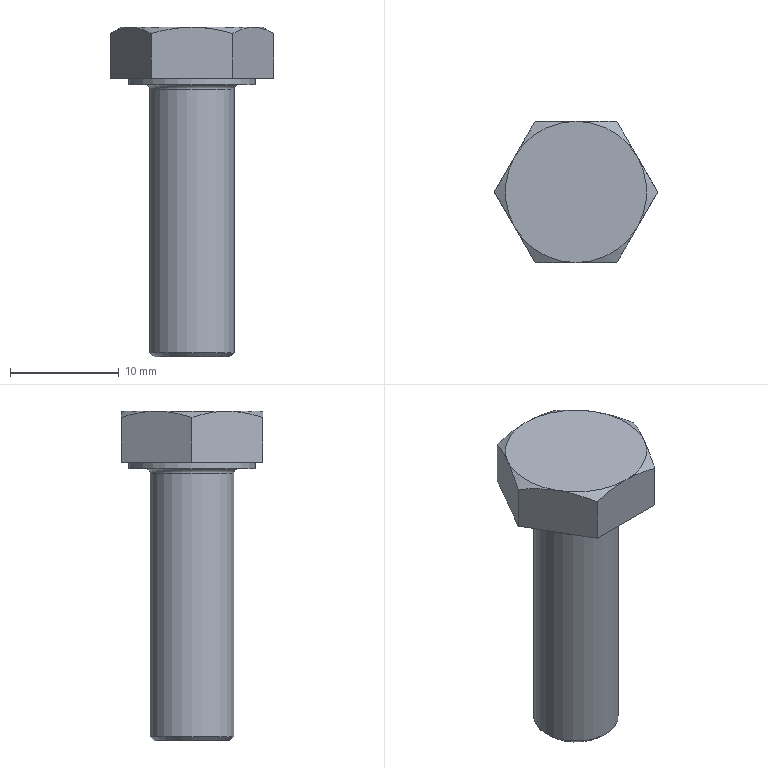Part | NX | 1 solid | 20 faces | box 15.011 x 13 x 30.3 mm | volume 1931 mm3 | plane 10 | cone 7 | cylinder 2 | torus 1 | commonest cylinder face diameters 7.76 x1 11.63 x1
STEP:
#1=CARTESIAN_POINT('',(3.753,-6.5,4.719));
#2=VERTEX_POINT('',#1);
#3=CARTESIAN_POINT('',(5.629,-3.25,5.3));
#4=VERTEX_POINT('',#3);
#5=CARTESIAN_POINT('',(3.753,-6.5,4.719));
#6=CARTESIAN_POINT('',(4.366,-5.438,5.073));
#7=CARTESIAN_POINT('',(4.989,-4.359,5.3));
#8=CARTESIAN_POINT('',(5.629,-3.25,5.3));
#9=B_SPLINE_CURVE_WITH_KNOTS('',3,(#5,#6,#7,#8),.UNSPECIFIED.,.F.,.F.,(4,4),(0.,1.),.UNSPECIFIED.);
#10=EDGE_CURVE('',#2,#4,#9,.T.);
#11=ORIENTED_EDGE('',*,*,#10,.F.);
#12=CARTESIAN_POINT('',(3.753,-6.5,0.6));
#13=VERTEX_POINT('',#12);
#14=CARTESIAN_POINT('',(3.753,-6.5,5.3));
#15=DIRECTION('',(0.,0.,-1.));
#16=VECTOR('',#15,1.);
#17=LINE('',#14,#16);
#18=EDGE_CURVE('',#2,#13,#17,.T.);
#19=ORIENTED_EDGE('',*,*,#18,.T.);
#20=CARTESIAN_POINT('',(7.506,0.,0.6));
#21=VERTEX_POINT('',#20);
#22=CARTESIAN_POINT('',(3.753,-6.5,0.6));
#23=DIRECTION('',(0.5,0.866,0.));
#24=VECTOR('',#23,1.);
#25=LINE('',#22,#24);
#26=EDGE_CURVE('',#13,#21,#25,.T.);
#27=ORIENTED_EDGE('',*,*,#26,.T.);
#28=CARTESIAN_POINT('',(7.506,0.,4.719));
#29=VERTEX_POINT('',#28);
#30=CARTESIAN_POINT('',(7.506,0.,5.3));
#31=DIRECTION('',(0.,0.,-1.));
#32=VECTOR('',#31,1.);
#33=LINE('',#30,#32);
#34=EDGE_CURVE('',#29,#21,#33,.T.);
#35=ORIENTED_EDGE('',*,*,#34,.F.);
#36=CARTESIAN_POINT('',(5.629,-3.25,5.3));
#37=CARTESIAN_POINT('',(6.27,-2.141,5.3));
#38=CARTESIAN_POINT('',(6.892,-1.062,5.073));
#39=CARTESIAN_POINT('',(7.506,0.,4.719));
#40=B_SPLINE_CURVE_WITH_KNOTS('',3,(#36,#37,#38,#39),.UNSPECIFIED.,.F.,.F.,(4,4),(0.,1.),.UNSPECIFIED.);
#41=EDGE_CURVE('',#4,#29,#40,.T.);
#42=ORIENTED_EDGE('',*,*,#41,.F.);
#43=EDGE_LOOP('',(#11,#19,#27,#35,#42));
#44=FACE_OUTER_BOUND('',#43,.T.);
#45=CARTESIAN_POINT('',(3.753,-6.5,5.3));
#46=DIRECTION('',(-0.866,0.5,0.));
#47=DIRECTION('',(0.5,0.866,0.));
#48=AXIS2_PLACEMENT_3D('',#45,#46,#47);
#49=PLANE('',#48);
#50=ADVANCED_FACE('',(#44),#49,.F.);
#51=CARTESIAN_POINT('',(5.629,3.25,5.3));
#52=VERTEX_POINT('',#51);
#53=CARTESIAN_POINT('',(7.506,0.,4.719));
#54=CARTESIAN_POINT('',(6.892,1.062,5.073));
#55=CARTESIAN_POINT('',(6.27,2.141,5.3));
#56=CARTESIAN_POINT('',(5.629,3.25,5.3));
#57=B_SPLINE_CURVE_WITH_KNOTS('',3,(#53,#54,#55,#56),.UNSPECIFIED.,.F.,.F.,(4,4),(0.,1.),.UNSPECIFIED.);
#58=EDGE_CURVE('',#29,#52,#57,.T.);
#59=ORIENTED_EDGE('',*,*,#58,.F.);
#60=ORIENTED_EDGE('',*,*,#34,.T.);
#61=CARTESIAN_POINT('',(3.753,6.5,0.6));
#62=VERTEX_POINT('',#61);
#63=CARTESIAN_POINT('',(7.506,0.,0.6));
#64=DIRECTION('',(-0.5,0.866,0.));
#65=VECTOR('',#64,1.);
#66=LINE('',#63,#65);
#67=EDGE_CURVE('',#21,#62,#66,.T.);
#68=ORIENTED_EDGE('',*,*,#67,.T.);
#69=CARTESIAN_POINT('',(3.753,6.5,4.719));
#70=VERTEX_POINT('',#69);
#71=CARTESIAN_POINT('',(3.753,6.5,5.3));
#72=DIRECTION('',(0.,0.,-1.));
#73=VECTOR('',#72,1.);
#74=LINE('',#71,#73);
#75=EDGE_CURVE('',#70,#62,#74,.T.);
#76=ORIENTED_EDGE('',*,*,#75,.F.);
#77=CARTESIAN_POINT('',(5.629,3.25,5.3));
#78=CARTESIAN_POINT('',(4.989,4.359,5.3));
#79=CARTESIAN_POINT('',(4.366,5.438,5.073));
#80=CARTESIAN_POINT('',(3.753,6.5,4.719));
#81=B_SPLINE_CURVE_WITH_KNOTS('',3,(#77,#78,#79,#80),.UNSPECIFIED.,.F.,.F.,(4,4),(0.,1.),.UNSPECIFIED.);
#82=EDGE_CURVE('',#52,#70,#81,.T.);
#83=ORIENTED_EDGE('',*,*,#82,.F.);
#84=EDGE_LOOP('',(#59,#60,#68,#76,#83));
#85=FACE_OUTER_BOUND('',#84,.T.);
#86=CARTESIAN_POINT('',(7.506,0.,5.3));
#87=DIRECTION('',(-0.866,-0.5,0.));
#88=DIRECTION('',(-0.5,0.866,0.));
#89=AXIS2_PLACEMENT_3D('',#86,#87,#88);
#90=PLANE('',#89);
#91=ADVANCED_FACE('',(#85),#90,.F.);
#92=CARTESIAN_POINT('',(0.,6.5,5.3));
#93=VERTEX_POINT('',#92);
#94=CARTESIAN_POINT('',(3.753,6.5,4.719));
#95=CARTESIAN_POINT('',(2.527,6.5,5.073));
#96=CARTESIAN_POINT('',(1.281,6.5,5.3));
#97=CARTESIAN_POINT('',(0.,6.5,5.3));
#98=B_SPLINE_CURVE_WITH_KNOTS('',3,(#94,#95,#96,#97),.UNSPECIFIED.,.F.,.F.,(4,4),(0.,1.),.UNSPECIFIED.);
#99=EDGE_CURVE('',#70,#93,#98,.T.);
#100=ORIENTED_EDGE('',*,*,#99,.F.);
#101=ORIENTED_EDGE('',*,*,#75,.T.);
#102=CARTESIAN_POINT('',(-3.753,6.5,0.6));
#103=VERTEX_POINT('',#102);
#104=CARTESIAN_POINT('',(3.753,6.5,0.6));
#105=DIRECTION('',(-1.,0.,0.));
#106=VECTOR('',#105,1.);
#107=LINE('',#104,#106);
#108=EDGE_CURVE('',#62,#103,#107,.T.);
#109=ORIENTED_EDGE('',*,*,#108,.T.);
#110=CARTESIAN_POINT('',(-3.753,6.5,4.719));
#111=VERTEX_POINT('',#110);
#112=CARTESIAN_POINT('',(-3.753,6.5,5.3));
#113=DIRECTION('',(0.,0.,-1.));
#114=VECTOR('',#113,1.);
#115=LINE('',#112,#114);
#116=EDGE_CURVE('',#111,#103,#115,.T.);
#117=ORIENTED_EDGE('',*,*,#116,.F.);
#118=CARTESIAN_POINT('',(0.,6.5,5.3));
#119=CARTESIAN_POINT('',(-1.281,6.5,5.3));
#120=CARTESIAN_POINT('',(-2.527,6.5,5.073));
#121=CARTESIAN_POINT('',(-3.753,6.5,4.719));
#122=B_SPLINE_CURVE_WITH_KNOTS('',3,(#118,#119,#120,#121),.UNSPECIFIED.,.F.,.F.,(4,4),(0.,1.),.UNSPECIFIED.);
#123=EDGE_CURVE('',#93,#111,#122,.T.);
#124=ORIENTED_EDGE('',*,*,#123,.F.);
#125=EDGE_LOOP('',(#100,#101,#109,#117,#124));
#126=FACE_OUTER_BOUND('',#125,.T.);
#127=CARTESIAN_POINT('',(3.753,6.5,5.3));
#128=DIRECTION('',(0.,-1.,0.));
#129=DIRECTION('',(-1.,0.,0.));
#130=AXIS2_PLACEMENT_3D('',#127,#128,#129);
#131=PLANE('',#130);
#132=ADVANCED_FACE('',(#126),#131,.F.);
#133=CARTESIAN_POINT('',(-5.629,3.25,5.3));
#134=VERTEX_POINT('',#133);
#135=CARTESIAN_POINT('',(-3.753,6.5,4.719));
#136=CARTESIAN_POINT('',(-4.366,5.438,5.073));
#137=CARTESIAN_POINT('',(-4.989,4.359,5.3));
#138=CARTESIAN_POINT('',(-5.629,3.25,5.3));
#139=B_SPLINE_CURVE_WITH_KNOTS('',3,(#135,#136,#137,#138),.UNSPECIFIED.,.F.,.F.,(4,4),(0.,1.),.UNSPECIFIED.);
#140=EDGE_CURVE('',#111,#134,#139,.T.);
#141=ORIENTED_EDGE('',*,*,#140,.F.);
#142=ORIENTED_EDGE('',*,*,#116,.T.);
#143=CARTESIAN_POINT('',(-7.506,0.,0.6));
#144=VERTEX_POINT('',#143);
#145=CARTESIAN_POINT('',(-3.753,6.5,0.6));
#146=DIRECTION('',(-0.5,-0.866,0.));
#147=VECTOR('',#146,1.);
#148=LINE('',#145,#147);
#149=EDGE_CURVE('',#103,#144,#148,.T.);
#150=ORIENTED_EDGE('',*,*,#149,.T.);
#151=CARTESIAN_POINT('',(-7.506,0.,4.719));
#152=VERTEX_POINT('',#151);
#153=CARTESIAN_POINT('',(-7.506,0.,5.3));
#154=DIRECTION('',(0.,0.,-1.));
#155=VECTOR('',#154,1.);
#156=LINE('',#153,#155);
#157=EDGE_CURVE('',#152,#144,#156,.T.);
#158=ORIENTED_EDGE('',*,*,#157,.F.);
#159=CARTESIAN_POINT('',(-5.629,3.25,5.3));
#160=CARTESIAN_POINT('',(-6.27,2.141,5.3));
#161=CARTESIAN_POINT('',(-6.892,1.062,5.073));
#162=CARTESIAN_POINT('',(-7.506,0.,4.719));
#163=B_SPLINE_CURVE_WITH_KNOTS('',3,(#159,#160,#161,#162),.UNSPECIFIED.,.F.,.F.,(4,4),(0.,1.),.UNSPECIFIED.);
#164=EDGE_CURVE('',#134,#152,#163,.T.);
#165=ORIENTED_EDGE('',*,*,#164,.F.);
#166=EDGE_LOOP('',(#141,#142,#150,#158,#165));
#167=FACE_OUTER_BOUND('',#166,.T.);
#168=CARTESIAN_POINT('',(-3.753,6.5,5.3));
#169=DIRECTION('',(0.866,-0.5,0.));
#170=DIRECTION('',(-0.5,-0.866,0.));
#171=AXIS2_PLACEMENT_3D('',#168,#169,#170);
#172=PLANE('',#171);
#173=ADVANCED_FACE('',(#167),#172,.F.);
#174=CARTESIAN_POINT('',(-5.629,-3.25,5.3));
#175=VERTEX_POINT('',#174);
#176=CARTESIAN_POINT('',(-7.506,0.,4.719));
#177=CARTESIAN_POINT('',(-6.892,-1.062,5.073));
#178=CARTESIAN_POINT('',(-6.27,-2.141,5.3));
#179=CARTESIAN_POINT('',(-5.629,-3.25,5.3));
#180=B_SPLINE_CURVE_WITH_KNOTS('',3,(#176,#177,#178,#179),.UNSPECIFIED.,.F.,.F.,(4,4),(0.,1.),.UNSPECIFIED.);
#181=EDGE_CURVE('',#152,#175,#180,.T.);
#182=ORIENTED_EDGE('',*,*,#181,.F.);
#183=ORIENTED_EDGE('',*,*,#157,.T.);
#184=CARTESIAN_POINT('',(-3.753,-6.5,0.6));
#185=VERTEX_POINT('',#184);
#186=CARTESIAN_POINT('',(-7.506,0.,0.6));
#187=DIRECTION('',(0.5,-0.866,0.));
#188=VECTOR('',#187,1.);
#189=LINE('',#186,#188);
#190=EDGE_CURVE('',#144,#185,#189,.T.);
#191=ORIENTED_EDGE('',*,*,#190,.T.);
#192=CARTESIAN_POINT('',(-3.753,-6.5,4.719));
#193=VERTEX_POINT('',#192);
#194=CARTESIAN_POINT('',(-3.753,-6.5,5.3));
#195=DIRECTION('',(0.,0.,-1.));
#196=VECTOR('',#195,1.);
#197=LINE('',#194,#196);
#198=EDGE_CURVE('',#193,#185,#197,.T.);
#199=ORIENTED_EDGE('',*,*,#198,.F.);
#200=CARTESIAN_POINT('',(-5.629,-3.25,5.3));
#201=CARTESIAN_POINT('',(-4.989,-4.359,5.3));
#202=CARTESIAN_POINT('',(-4.366,-5.438,5.073));
#203=CARTESIAN_POINT('',(-3.753,-6.5,4.719));
#204=B_SPLINE_CURVE_WITH_KNOTS('',3,(#200,#201,#202,#203),.UNSPECIFIED.,.F.,.F.,(4,4),(0.,1.),.UNSPECIFIED.);
#205=EDGE_CURVE('',#175,#193,#204,.T.);
#206=ORIENTED_EDGE('',*,*,#205,.F.);
#207=EDGE_LOOP('',(#182,#183,#191,#199,#206));
#208=FACE_OUTER_BOUND('',#207,.T.);
#209=CARTESIAN_POINT('',(-7.506,0.,5.3));
#210=DIRECTION('',(0.866,0.5,0.));
#211=DIRECTION('',(0.5,-0.866,0.));
#212=AXIS2_PLACEMENT_3D('',#209,#210,#211);
#213=PLANE('',#212);
#214=ADVANCED_FACE('',(#208),#213,.F.);
#215=CARTESIAN_POINT('',(0.,-6.5,5.3));
#216=VERTEX_POINT('',#215);
#217=CARTESIAN_POINT('',(-3.753,-6.5,4.719));
#218=CARTESIAN_POINT('',(-2.527,-6.5,5.073));
#219=CARTESIAN_POINT('',(-1.281,-6.5,5.3));
#220=CARTESIAN_POINT('',(0.,-6.5,5.3));
#221=B_SPLINE_CURVE_WITH_KNOTS('',3,(#217,#218,#219,#220),.UNSPECIFIED.,.F.,.F.,(4,4),(0.,1.),.UNSPECIFIED.);
#222=EDGE_CURVE('',#193,#216,#221,.T.);
#223=ORIENTED_EDGE('',*,*,#222,.F.);
#224=ORIENTED_EDGE('',*,*,#198,.T.);
#225=CARTESIAN_POINT('',(-3.753,-6.5,0.6));
#226=DIRECTION('',(1.,0.,0.));
#227=VECTOR('',#226,1.);
#228=LINE('',#225,#227);
#229=EDGE_CURVE('',#185,#13,#228,.T.);
#230=ORIENTED_EDGE('',*,*,#229,.T.);
#231=ORIENTED_EDGE('',*,*,#18,.F.);
#232=CARTESIAN_POINT('',(0.,-6.5,5.3));
#233=CARTESIAN_POINT('',(1.281,-6.5,5.3));
#234=CARTESIAN_POINT('',(2.527,-6.5,5.073));
#235=CARTESIAN_POINT('',(3.753,-6.5,4.719));
#236=B_SPLINE_CURVE_WITH_KNOTS('',3,(#232,#233,#234,#235),.UNSPECIFIED.,.F.,.F.,(4,4),(0.,1.),.UNSPECIFIED.);
#237=EDGE_CURVE('',#216,#2,#236,.T.);
#238=ORIENTED_EDGE('',*,*,#237,.F.);
#239=EDGE_LOOP('',(#223,#224,#230,#231,#238));
#240=FACE_OUTER_BOUND('',#239,.T.);
#241=CARTESIAN_POINT('',(-3.753,-6.5,5.3));
#242=DIRECTION('',(0.,1.,0.));
#243=DIRECTION('',(1.,0.,0.));
#244=AXIS2_PLACEMENT_3D('',#241,#242,#243);
#245=PLANE('',#244);
#246=ADVANCED_FACE('',(#240),#245,.F.);
#247=CARTESIAN_POINT('',(5.815,0.,0.6));
#248=VERTEX_POINT('',#247);
#249=CARTESIAN_POINT('',(0.,0.,0.6));
#250=DIRECTION('',(0.,0.,1.));
#251=DIRECTION('',(1.,0.,0.));
#252=AXIS2_PLACEMENT_3D('',#249,#250,#251);
#253=CIRCLE('',#252,5.815);
#254=EDGE_CURVE('',#248,#248,#253,.T.);
#255=ORIENTED_EDGE('',*,*,#254,.T.);
#256=EDGE_LOOP('',(#255));
#257=FACE_BOUND('',#256,.T.);
#258=ORIENTED_EDGE('',*,*,#26,.F.);
#259=ORIENTED_EDGE('',*,*,#229,.F.);
#260=ORIENTED_EDGE('',*,*,#190,.F.);
#261=ORIENTED_EDGE('',*,*,#149,.F.);
#262=ORIENTED_EDGE('',*,*,#108,.F.);
#263=ORIENTED_EDGE('',*,*,#67,.F.);
#264=EDGE_LOOP('',(#258,#259,#260,#261,#262,#263));
#265=FACE_BOUND('',#264,.T.);
#266=CARTESIAN_POINT('',(11.258,6.5,0.6));
#267=DIRECTION('',(0.,0.,1.));
#268=DIRECTION('',(-1.,0.,0.));
#269=AXIS2_PLACEMENT_3D('',#266,#267,#268);
#270=PLANE('',#269);
#271=ADVANCED_FACE('',(#257,#265),#270,.F.);
#272=ORIENTED_EDGE('',*,*,#10,.T.);
#273=CARTESIAN_POINT('',(0.,0.,5.3));
#274=DIRECTION('',(0.,0.,-1.));
#275=DIRECTION('',(-1.,0.,0.));
#276=AXIS2_PLACEMENT_3D('',#273,#274,#275);
#277=CIRCLE('',#276,6.5);
#278=EDGE_CURVE('',#4,#216,#277,.T.);
#279=ORIENTED_EDGE('',*,*,#278,.T.);
#280=ORIENTED_EDGE('',*,*,#237,.T.);
#281=EDGE_LOOP('',(#272,#279,#280));
#282=FACE_OUTER_BOUND('',#281,.T.);
#283=CARTESIAN_POINT('',(0.,0.,4.719));
#284=DIRECTION('',(0.,0.,-1.));
#285=DIRECTION('',(1.,0.,0.));
#286=AXIS2_PLACEMENT_3D('',#283,#284,#285);
#287=CONICAL_SURFACE('',#286,7.506,60.);
#288=ADVANCED_FACE('',(#282),#287,.T.);
#289=ORIENTED_EDGE('',*,*,#205,.T.);
#290=ORIENTED_EDGE('',*,*,#222,.T.);
#291=CARTESIAN_POINT('',(0.,0.,5.3));
#292=DIRECTION('',(0.,0.,-1.));
#293=DIRECTION('',(-1.,0.,0.));
#294=AXIS2_PLACEMENT_3D('',#291,#292,#293);
#295=CIRCLE('',#294,6.5);
#296=EDGE_CURVE('',#216,#175,#295,.T.);
#297=ORIENTED_EDGE('',*,*,#296,.T.);
#298=EDGE_LOOP('',(#289,#290,#297));
#299=FACE_OUTER_BOUND('',#298,.T.);
#300=CARTESIAN_POINT('',(0.,0.,4.719));
#301=DIRECTION('',(0.,0.,-1.));
#302=DIRECTION('',(1.,0.,0.));
#303=AXIS2_PLACEMENT_3D('',#300,#301,#302);
#304=CONICAL_SURFACE('',#303,7.506,60.);
#305=ADVANCED_FACE('',(#299),#304,.T.);
#306=ORIENTED_EDGE('',*,*,#164,.T.);
#307=ORIENTED_EDGE('',*,*,#181,.T.);
#308=CARTESIAN_POINT('',(0.,0.,5.3));
#309=DIRECTION('',(0.,0.,-1.));
#310=DIRECTION('',(-1.,0.,0.));
#311=AXIS2_PLACEMENT_3D('',#308,#309,#310);
#312=CIRCLE('',#311,6.5);
#313=EDGE_CURVE('',#175,#134,#312,.T.);
#314=ORIENTED_EDGE('',*,*,#313,.T.);
#315=EDGE_LOOP('',(#306,#307,#314));
#316=FACE_OUTER_BOUND('',#315,.T.);
#317=CARTESIAN_POINT('',(0.,0.,4.719));
#318=DIRECTION('',(0.,0.,-1.));
#319=DIRECTION('',(1.,0.,0.));
#320=AXIS2_PLACEMENT_3D('',#317,#318,#319);
#321=CONICAL_SURFACE('',#320,7.506,60.);
#322=ADVANCED_FACE('',(#316),#321,.T.);
#323=ORIENTED_EDGE('',*,*,#123,.T.);
#324=ORIENTED_EDGE('',*,*,#140,.T.);
#325=CARTESIAN_POINT('',(0.,0.,5.3));
#326=DIRECTION('',(0.,0.,-1.));
#327=DIRECTION('',(-1.,0.,0.));
#328=AXIS2_PLACEMENT_3D('',#325,#326,#327);
#329=CIRCLE('',#328,6.5);
#330=EDGE_CURVE('',#134,#93,#329,.T.);
#331=ORIENTED_EDGE('',*,*,#330,.T.);
#332=EDGE_LOOP('',(#323,#324,#331));
#333=FACE_OUTER_BOUND('',#332,.T.);
#334=CARTESIAN_POINT('',(0.,0.,4.719));
#335=DIRECTION('',(0.,0.,-1.));
#336=DIRECTION('',(1.,0.,0.));
#337=AXIS2_PLACEMENT_3D('',#334,#335,#336);
#338=CONICAL_SURFACE('',#337,7.506,60.);
#339=ADVANCED_FACE('',(#333),#338,.T.);
#340=ORIENTED_EDGE('',*,*,#82,.T.);
#341=ORIENTED_EDGE('',*,*,#99,.T.);
#342=CARTESIAN_POINT('',(0.,0.,5.3));
#343=DIRECTION('',(0.,0.,-1.));
#344=DIRECTION('',(-1.,0.,0.));
#345=AXIS2_PLACEMENT_3D('',#342,#343,#344);
#346=CIRCLE('',#345,6.5);
#347=EDGE_CURVE('',#93,#52,#346,.T.);
#348=ORIENTED_EDGE('',*,*,#347,.T.);
#349=EDGE_LOOP('',(#340,#341,#348));
#350=FACE_OUTER_BOUND('',#349,.T.);
#351=CARTESIAN_POINT('',(0.,0.,4.719));
#352=DIRECTION('',(0.,0.,-1.));
#353=DIRECTION('',(1.,0.,0.));
#354=AXIS2_PLACEMENT_3D('',#351,#352,#353);
#355=CONICAL_SURFACE('',#354,7.506,60.);
#356=ADVANCED_FACE('',(#350),#355,.T.);
#357=ORIENTED_EDGE('',*,*,#41,.T.);
#358=ORIENTED_EDGE('',*,*,#58,.T.);
#359=CARTESIAN_POINT('',(0.,0.,5.3));
#360=DIRECTION('',(0.,0.,-1.));
#361=DIRECTION('',(-1.,0.,0.));
#362=AXIS2_PLACEMENT_3D('',#359,#360,#361);
#363=CIRCLE('',#362,6.5);
#364=EDGE_CURVE('',#52,#4,#363,.T.);
#365=ORIENTED_EDGE('',*,*,#364,.T.);
#366=EDGE_LOOP('',(#357,#358,#365));
#367=FACE_OUTER_BOUND('',#366,.T.);
#368=CARTESIAN_POINT('',(0.,0.,4.719));
#369=DIRECTION('',(0.,0.,-1.));
#370=DIRECTION('',(1.,0.,0.));
#371=AXIS2_PLACEMENT_3D('',#368,#369,#370);
#372=CONICAL_SURFACE('',#371,7.506,60.);
#373=ADVANCED_FACE('',(#367),#372,.T.);
#374=ORIENTED_EDGE('',*,*,#330,.F.);
#375=ORIENTED_EDGE('',*,*,#313,.F.);
#376=ORIENTED_EDGE('',*,*,#296,.F.);
#377=ORIENTED_EDGE('',*,*,#278,.F.);
#378=ORIENTED_EDGE('',*,*,#364,.F.);
#379=ORIENTED_EDGE('',*,*,#347,.F.);
#380=EDGE_LOOP('',(#374,#375,#376,#377,#378,#379));
#381=FACE_OUTER_BOUND('',#380,.T.);
#382=CARTESIAN_POINT('',(11.258,6.5,5.3));
#383=DIRECTION('',(0.,0.,1.));
#384=DIRECTION('',(-1.,0.,0.));
#385=AXIS2_PLACEMENT_3D('',#382,#383,#384);
#386=PLANE('',#385);
#387=ADVANCED_FACE('',(#381),#386,.T.);
#388=ORIENTED_EDGE('',*,*,#254,.F.);
#389=EDGE_LOOP('',(#388));
#390=FACE_BOUND('',#389,.T.);
#391=CARTESIAN_POINT('',(5.815,0.,0.));
#392=VERTEX_POINT('',#391);
#393=CARTESIAN_POINT('',(0.,0.,0.));
#394=DIRECTION('',(0.,0.,1.));
#395=DIRECTION('',(1.,0.,0.));
#396=AXIS2_PLACEMENT_3D('',#393,#394,#395);
#397=CIRCLE('',#396,5.815);
#398=EDGE_CURVE('',#392,#392,#397,.T.);
#399=ORIENTED_EDGE('',*,*,#398,.T.);
#400=EDGE_LOOP('',(#399));
#401=FACE_BOUND('',#400,.T.);
#402=CARTESIAN_POINT('',(0.,0.,0.6));
#403=DIRECTION('',(0.,0.,-1.));
#404=DIRECTION('',(1.,0.,0.));
#405=AXIS2_PLACEMENT_3D('',#402,#403,#404);
#406=CYLINDRICAL_SURFACE('',#405,5.815);
#407=ADVANCED_FACE('',(#390,#401),#406,.T.);
#408=CARTESIAN_POINT('',(4.28,0.,0.));
#409=VERTEX_POINT('',#408);
#410=CARTESIAN_POINT('',(0.,0.,0.));
#411=DIRECTION('',(0.,0.,1.));
#412=DIRECTION('',(1.,0.,0.));
#413=AXIS2_PLACEMENT_3D('',#410,#411,#412);
#414=CIRCLE('',#413,4.28);
#415=EDGE_CURVE('',#409,#409,#414,.T.);
#416=ORIENTED_EDGE('',*,*,#415,.T.);
#417=EDGE_LOOP('',(#416));
#418=FACE_BOUND('',#417,.T.);
#419=ORIENTED_EDGE('',*,*,#398,.F.);
#420=EDGE_LOOP('',(#419));
#421=FACE_BOUND('',#420,.T.);
#422=CARTESIAN_POINT('',(0.,0.,0.));
#423=DIRECTION('',(0.,0.,1.));
#424=DIRECTION('',(-1.,0.,0.));
#425=AXIS2_PLACEMENT_3D('',#422,#423,#424);
#426=PLANE('',#425);
#427=ADVANCED_FACE('',(#418,#421),#426,.F.);
#428=CARTESIAN_POINT('',(3.88,0.,-0.4));
#429=VERTEX_POINT('',#428);
#430=CARTESIAN_POINT('',(0.,0.,-0.4));
#431=DIRECTION('',(0.,0.,-1.));
#432=DIRECTION('',(1.,0.,0.));
#433=AXIS2_PLACEMENT_3D('',#430,#431,#432);
#434=CIRCLE('',#433,3.88);
#435=EDGE_CURVE('',#429,#429,#434,.T.);
#436=ORIENTED_EDGE('',*,*,#435,.T.);
#437=EDGE_LOOP('',(#436));
#438=FACE_BOUND('',#437,.T.);
#439=CARTESIAN_POINT('',(3.88,0.,-24.612));
#440=VERTEX_POINT('',#439);
#441=CARTESIAN_POINT('',(0.,0.,-24.612));
#442=DIRECTION('',(0.,0.,1.));
#443=DIRECTION('',(1.,0.,0.));
#444=AXIS2_PLACEMENT_3D('',#441,#442,#443);
#445=CIRCLE('',#444,3.88);
#446=EDGE_CURVE('',#440,#440,#445,.T.);
#447=ORIENTED_EDGE('',*,*,#446,.T.);
#448=EDGE_LOOP('',(#447));
#449=FACE_BOUND('',#448,.T.);
#450=CARTESIAN_POINT('',(0.,0.,-25.));
#451=DIRECTION('',(0.,0.,1.));
#452=DIRECTION('',(-1.,0.,0.));
#453=AXIS2_PLACEMENT_3D('',#450,#451,#452);
#454=CYLINDRICAL_SURFACE('',#453,3.88);
#455=ADVANCED_FACE('',(#438,#449),#454,.T.);
#456=CARTESIAN_POINT('',(3.492,0.,-25.));
#457=VERTEX_POINT('',#456);
#458=CARTESIAN_POINT('',(0.,0.,-25.));
#459=DIRECTION('',(0.,0.,-1.));
#460=DIRECTION('',(1.,0.,0.));
#461=AXIS2_PLACEMENT_3D('',#458,#459,#460);
#462=CIRCLE('',#461,3.492);
#463=EDGE_CURVE('',#457,#457,#462,.T.);
#464=ORIENTED_EDGE('',*,*,#463,.T.);
#465=EDGE_LOOP('',(#464));
#466=FACE_OUTER_BOUND('',#465,.T.);
#467=CARTESIAN_POINT('',(0.,0.,-25.));
#468=DIRECTION('',(0.,0.,1.));
#469=DIRECTION('',(-1.,0.,0.));
#470=AXIS2_PLACEMENT_3D('',#467,#468,#469);
#471=PLANE('',#470);
#472=ADVANCED_FACE('',(#466),#471,.F.);
#473=ORIENTED_EDGE('',*,*,#463,.F.);
#474=EDGE_LOOP('',(#473));
#475=FACE_BOUND('',#474,.T.);
#476=ORIENTED_EDGE('',*,*,#446,.F.);
#477=EDGE_LOOP('',(#476));
#478=FACE_BOUND('',#477,.T.);
#479=CARTESIAN_POINT('',(0.,0.,-24.612));
#480=DIRECTION('',(0.,0.,1.));
#481=DIRECTION('',(-1.,0.,0.));
#482=AXIS2_PLACEMENT_3D('',#479,#480,#481);
#483=CONICAL_SURFACE('',#482,3.88,45.);
#484=ADVANCED_FACE('',(#475,#478),#483,.T.);
#485=ORIENTED_EDGE('',*,*,#435,.F.);
#486=EDGE_LOOP('',(#485));
#487=FACE_BOUND('',#486,.T.);
#488=ORIENTED_EDGE('',*,*,#415,.F.);
#489=EDGE_LOOP('',(#488));
#490=FACE_BOUND('',#489,.T.);
#491=CARTESIAN_POINT('',(0.,0.,-0.4));
#492=DIRECTION('',(0.,0.,1.));
#493=DIRECTION('',(-1.,0.,0.));
#494=AXIS2_PLACEMENT_3D('',#491,#492,#493);
#495=TOROIDAL_SURFACE('',#494,4.28,0.4);
#496=ADVANCED_FACE('',(#487,#490),#495,.F.);
#497=CLOSED_SHELL('',(#50,#91,#132,#173,#214,#246,#271,#288,#305,#322,#339,#356,#373,#387,#407,#427,#455,#472,#484,#496));
#498=MANIFOLD_SOLID_BREP('',#497);
#499=(LENGTH_UNIT()NAMED_UNIT(*)SI_UNIT(.MILLI.,.METRE.));
#500=UNCERTAINTY_MEASURE_WITH_UNIT(LENGTH_MEASURE(0.0508),#499,'','');
#501=(NAMED_UNIT(*)PLANE_ANGLE_UNIT()SI_UNIT($,.RADIAN.));
#502=PLANE_ANGLE_MEASURE_WITH_UNIT(PLANE_ANGLE_MEASURE(0.01745),#501);
#503=DIMENSIONAL_EXPONENTS(0.,0.,0.,0.,0.,0.,0.);
#504=(CONVERSION_BASED_UNIT('DEGREE',#502)NAMED_UNIT(#503)PLANE_ANGLE_UNIT());
#505=(NAMED_UNIT(*)SI_UNIT($,.STERADIAN.)SOLID_ANGLE_UNIT());
#506=(GEOMETRIC_REPRESENTATION_CONTEXT(3)GLOBAL_UNCERTAINTY_ASSIGNED_CONTEXT((#500))GLOBAL_UNIT_ASSIGNED_CONTEXT((#499,#504,#505))REPRESENTATION_CONTEXT('',''));
#507=ADVANCED_BREP_SHAPE_REPRESENTATION('',(#498),#506);